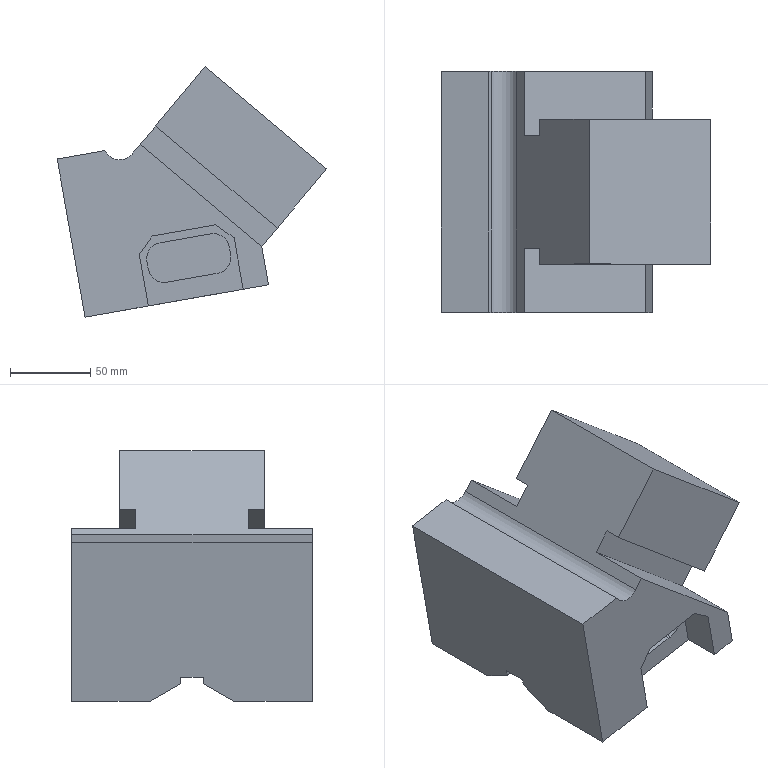Part | NX | features solid 2 | 1 solid | 57 faces | box 167.918 x 150 x 155.838 mm | volume 1697917 mm3 | plane 48 | cylinder 9 | commonest cylinder face diameters 20 x9